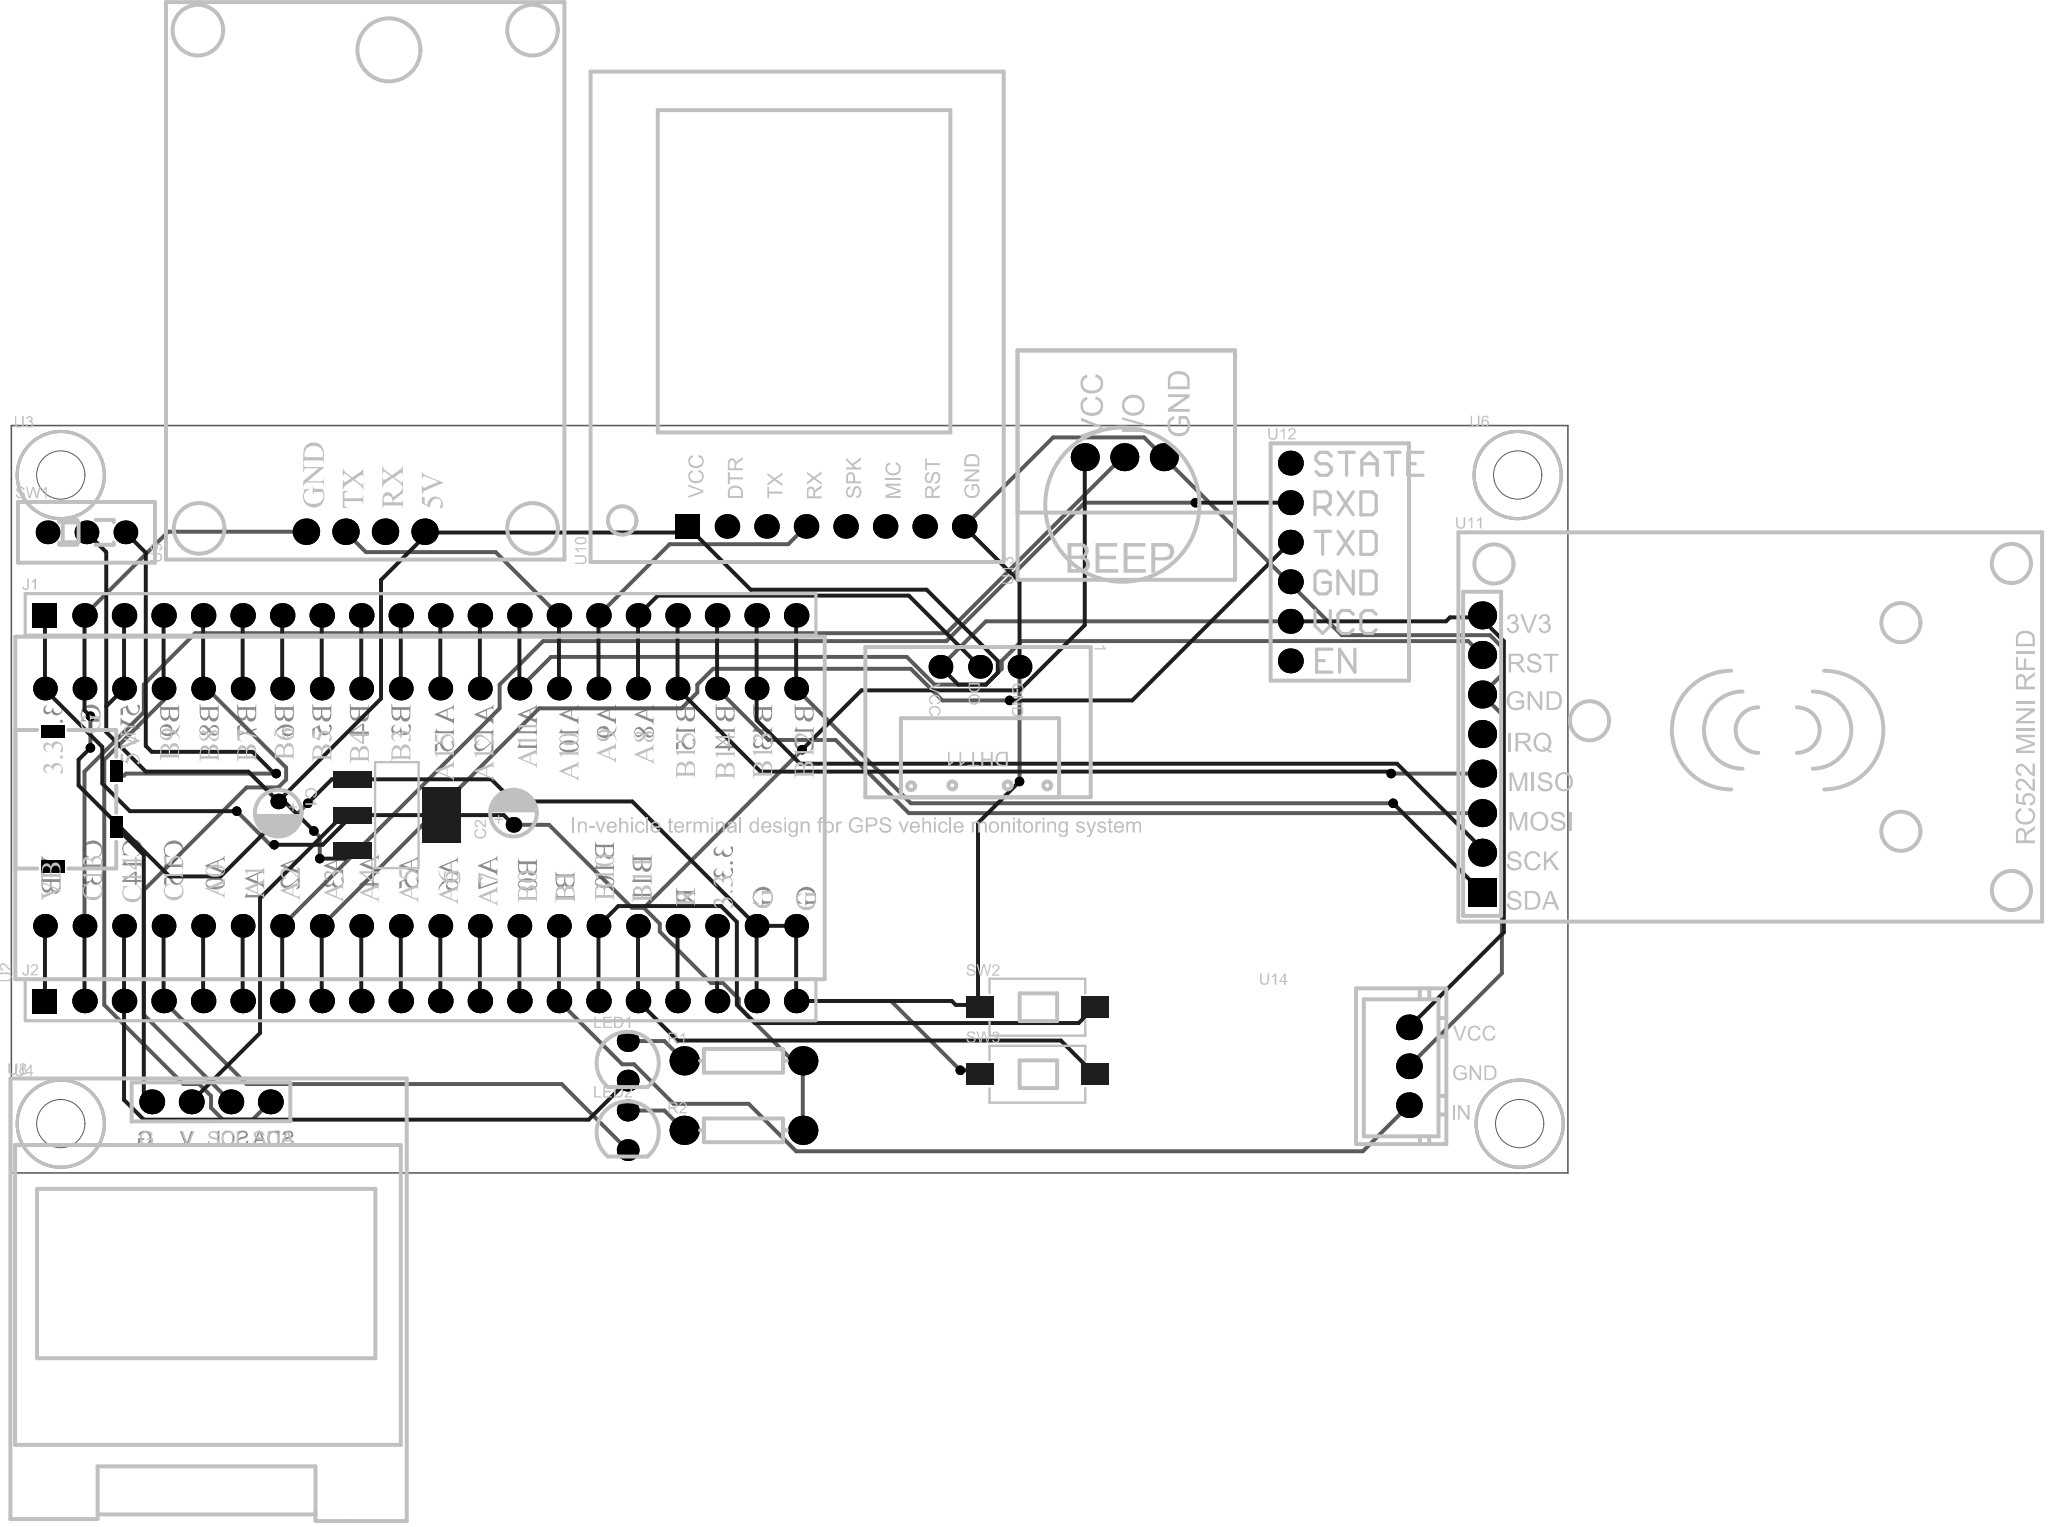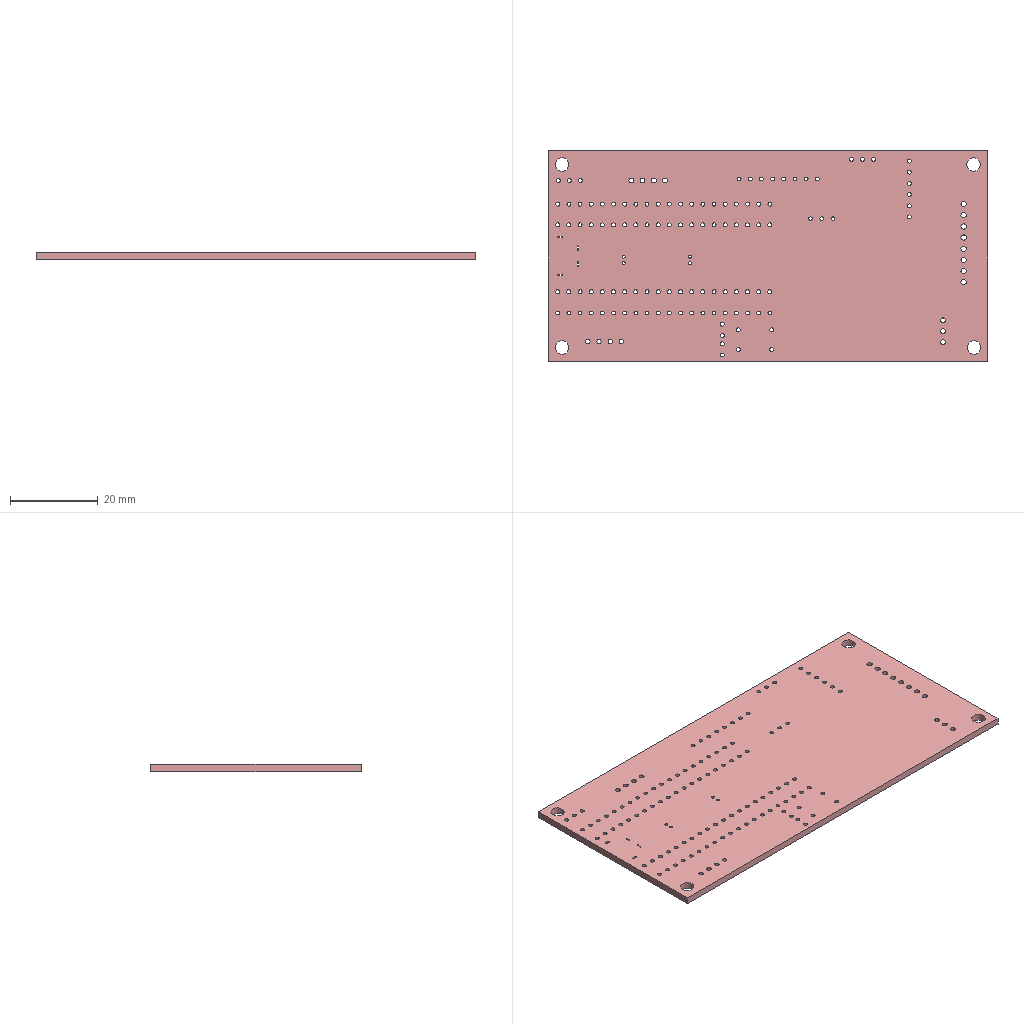Circuit board layout | Altium Designer | box 100 x 48 x 1.6 mm
Layer stack:
# Altium Designer layer stack of  (unit mm; dielectric type: 0 none, 1 core, 2 prepreg, 3 surface material)
index,name,kind,layer,copper_thickness_mm,dielectric_type,dielectric_thickness_mm,dielectric_material,dielectric_constant
0,Top Paste Mask Layer,other,,,,,,
1,Top Silkscreen Layer,other,,,,,,
2,Top Solder Mask Layer,dielectric,,,3,0.01,,3.3
3,Top Layer,copper,Top Layer,0.035,,,,
4,Dielectric1,dielectric,,,3,1.51,FR4,4.5
5,Bottom Layer,copper,Bottom Layer,0.035,,,,
6,Bottom Solder Mask Layer,dielectric,,,3,0.01,,3.3
7,Bottom Silkscreen Layer,other,,,,,,
8,Bottom Paste Mask Layer,other,,,,,,
# drill layer pairs: low layer,high layer
drill_pair,Top Layer,Bottom Layer
Part placement:
Designator,Comment,Layer,Footprint,Center-X(mm),Center-Y(mm),Rotation
C1,1u,TopLayer,CAP-D3.0¡ÁF1.5,103.854,121.666,270
C2,1u,TopLayer,CAP-D3.0¡ÁF1.5,118.967,121.666,90
J1,HDR-M-2.54_1x20,TopLayer,HDR-M-2.54_1X20,112.998,134.366,0
J2,HDR-M-2.54_1x20,TopLayer,HDR-M-2.54_1X20,112.998,109.601,0
SW1,SS12D00G3,TopLayer,SW-TH_SS-12D01-GX,91.535,139.7,0
U2,,TopLayer,FYS_STM32F103C最小系统,112.998,122.047,90
U4,Standoff,TopLayer,M3铜柱,0,0,0
U6,Standoff,TopLayer,M3铜柱,0,0,0
U5,Standoff,TopLayer,M3铜柱,0,0,0
U3,Standoff,TopLayer,M3铜柱,0,0,0
U7,TYPE-C 2P 90 2J 108,TopLayer,usb-a-th_type-c-2p-90-2j-108,91.408,122.555,270
U1,AMS1117-3.3,TopLayer,SOT-223_L6.5-W3.5-P2.30-LS7.0-BR,111.474,121.539,180
U8,FYS#0.96 OLED IIC_4PIN COPY COPY COPY,TopLayer,FYS_OLED_IIC,99.536,103.124,0
U9,FYS#GPS-6M_no mounting hole,TopLayer,FYS#GPS模块_不带槽,109.445,139.74,90
U10,FYS#SIM900AMINI,TopLayer,FYS#SIM900AMINI,139.033,140.081,90
U11,FYS#RC522 MINI RFID module COPY COPY,TopLayer,FYS#RC522_MINI_RFIDÄ£¿é_COPY_1,181.197,125.476,0
U13,FYS#BEEP buzzer module COPY,TopLayer,FYS#BEEP·äÃùÆ÷Ä£¿é_COPY,158.21,144.526,90
R2,1k,TopLayer,R_AXIAL-0.3,133.744,101.295,0
LED1,LED-TH-3mm_R,TopLayer,LED-TH_BD3.0_RED,126.306,105.758,0
LED2,LED-TH-3mm_R,TopLayer,LED-TH_BD3.0_RED,126.306,101.295,0
R1,1k,TopLayer,R_AXIAL-0.3,133.744,105.758,0
1,FYS#DHT11 COPY,TopLayer,FYS#DHT11_X_COPY,148.939,131.064,270
U12,FYS#HC series Bluetooth module COPY,TopLayer,FYS#HC-05À¶ÑÀÄ£¿é_COPY,168.878,137.795,0
U14,FYS#1-channel 5V optocoupler isolated relay module COPY,TopLayer,FYS#1Â·5V¹âÅ¼¸ôÀë¼ÌµçÆ÷Ä£¿é_COPY,176.498,105.41,0
SW2,1TS002B-2300-5001,TopLayer,SW-SMD_L6.0-W3.5-LS8.0,152.627,109.202,0
SW3,1TS002B-2300-5001,TopLayer,SW-SMD_L6.0-W3.5-LS8.0,152.627,104.897,0
Pad and via stacks:
# Altium Designer via and pad stacks of  (unit mm). Each distinct definition once, with the count of objects using it.
# via: kind,start_layer,end_layer,hole_mm,diameter_mm,mode(0 simple;1 top-mid-bottom;2 full stack),diameter_per_layer,count,example_net
# pad: kind,layer,hole_mm,hole_type(0 round;1 square;2 slot),plating,top_size,top_shape(1 round;2 rect;3 octagon;9 rounded rect),mid_size,bottom_size,mode,footprint,size_per_layer,count,example
pad,Multi-Layer,0.7,0,plated,1x1,1,1x1,1x1,0,CAP-D3.0\u00A1\u00C1F1.5,,4,C1.2
pad,Multi-Layer,0.889,0,plated,1.575x1.575,1,1.575x1.575,1.575x1.575,0,HDR-M-2.54_1X20,,38,J1.20
pad,Multi-Layer,0.889,0,plated,1.575x1.575,2,1.575x1.575,1.575x1.575,0,HDR-M-2.54_1X20,,2,J1.1
pad,Multi-Layer,0.9144,0,plated,1.524x1.524,1,1.524x1.524,1.524x1.524,0,SW-TH_SS-12D01-GX,,3,SW1.1
pad,Multi-Layer,0.9144,0,plated,1.524x1.524,1,1.524x1.524,1.524x1.524,0,FYS_STM32F103C\u00D7\u00EE\u00D0\u00A1\u00CF\u00B5\u00CD\u00B3,,40,U2.21
pad,Multi-Layer,0.36,2,plated,0.8x1.4,2,0.8x1.4,0.8x1.4,0,usb-a-th_type-c-2p-90-2j-108,,2,U7.2
pad,Multi-Layer,0.4,2,plated,0.8x1.524,2,0.8x1.524,0.8x1.524,0,usb-a-th_type-c-2p-90-2j-108,,2,U7.4
pad,Multi-Layer,1,2,plated,1.6x1.6,1,1.6x1.6,1.6x1.6,0,FYS_OLED_IIC,,4,U8.3
pad,Multi-Layer,1.1,2,plated,1.7x1.7,1,1.7x1.7,1.7x1.7,0,FYS#GPS\u00C4\u00A3\u00BF\u00E9_\u00B2\u00BB\u00B4\u00F8\u00B2\u00DB,,4,U9.3
pad,Multi-Layer,0.889,0,plated,1.575x1.575,2,1.575x1.575,1.575x1.575,0,FYS#SIM900AMINI,,1,U10.1
pad,Multi-Layer,0.889,0,plated,1.575x1.575,1,1.575x1.575,1.575x1.575,0,FYS#SIM900AMINI,,7,U10.2
pad,Multi-Layer,1.2,0,plated,1.8x1.8,1,1.8x1.8,1.8x1.8,0,FYS#RC522 MINI RFID\u00C4\u00A3\u00BF\u00E9 COPY_1,,7,U11.8
pad,Multi-Layer,1.2,0,plated,1.8x1.8,2,1.8x1.8,1.8x1.8,0,FYS#RC522 MINI RFID\u00C4\u00A3\u00BF\u00E9 COPY_1,,1,U11.1
pad,Multi-Layer,0.9002,2,plated,1.8x1.8,1,1.8x1.8,1.8x1.8,0,FYS#BEEP\u00B7\u00E4\u00C3\u00F9\u00C6\u00F7\u00C4\u00A3\u00BF\u00E9 COPY,,3,U13.3
pad,Multi-Layer,0.8992,0,plated,1.88x1.88,1,1.88x1.88,1.88x1.88,0,R_AXIAL-0.3,,4,R2.1
pad,Multi-Layer,0.9,0,plated,1.4x1.4,1,1.4x1.4,1.4x1.4,0,LED-TH_BD3.0_RED,,4,LED1.1
pad,Multi-Layer,0.81,2,plated,1.524x1.524,1,1.524x1.524,1.524x1.524,0,FYS#DHT11_X COPY,,3,1.1
pad,Multi-Layer,0.9,2,plated,1.6x1.6,1,1.6x1.6,1.6x1.6,0,FYS#HC-05\u00C0\u00B6\u00D1\u00C0\u00C4\u00A3\u00BF\u00E9 COPY,,6,U12.1
pad,Multi-Layer,1.1,0,plated,1.65x1.65,1,1.65x1.65,1.65x1.65,0,FYS#1\u00C2\u00B75V\u00B9\u00E2\u00C5\u00BC\u00B8\u00F4\u00C0\u00EB\u00BC\u00CC\u00B5\u00E7\u00C6\u00F7\u00C4\u00A3\u00BF\u00E9 COPY,,3,U14.3
pad,Top Layer,0,0,plated,2.465x1.05,2,2.465x1.05,2.465x1.05,0,SOT-223_L6.5-W3.5-P2.30-LS7.0-BR,,3,U1.1
pad,Top Layer,0,0,plated,2.465x3.54,2,2.465x3.54,2.465x3.54,0,SOT-223_L6.5-W3.5-P2.30-LS7.0-BR,,1,U1.4
pad,Top Layer,0,0,plated,1.74x1.4,2,1.74x1.4,1.74x1.4,0,SW-SMD_L6.0-W3.5-LS8.0,,4,SW2.1
via,Top Layer,Bottom Layer,0.3048,0.61,0,,16,GND